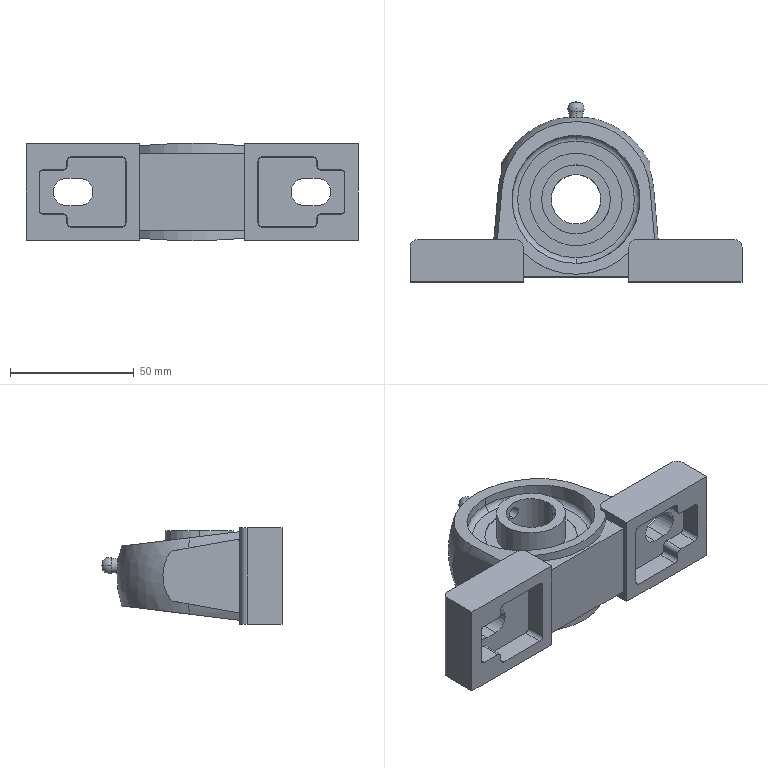Part | SolidWorks | features Revolution 5, Cut 3, Boss 2, CirPattern 2, ICE 2, RevCut 2, Extrusion 1, RefAxis 1, SweepCut 1 | 1 solid | 156 faces | box 134 x 72.66 x 39.214 mm | volume 104404 mm3 | plane 56 | cylinder 43 | sphere 28 | cone 16 | torus 8 | spline 5 | commonest cylinder face diameters 2 x6 6 x6 27.83 x6 37.32 x6 51.695 x6 5.134 x4